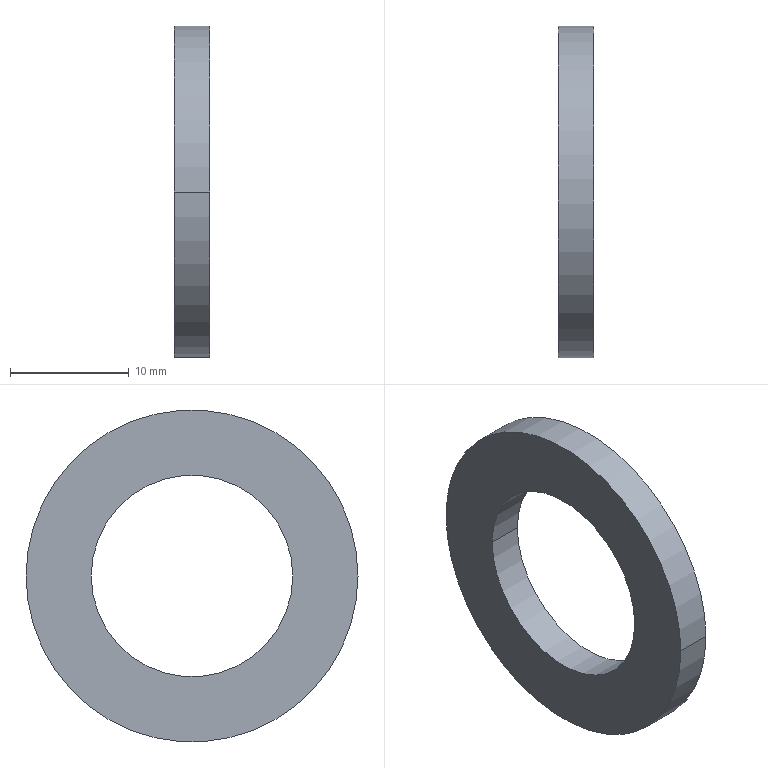Part | STEP file | KS B 1326 - 16x28 | 1 solid | 6 faces | box 3 x 28 x 28 mm | volume 1166 mm3 | cylinder 4 | plane 2 | commonest cylinder face diameters 17 x2 28 x2
STEP:
#1=CARTESIAN_POINT('',(0.,0.,0.));
#2=DIRECTION('',(0.,0.,1.));
#3=DIRECTION('',(1.,0.,0.));
#4=AXIS2_PLACEMENT_3D('',#1,#2,#3);
#5=CARTESIAN_POINT('',(0.,-8.5,0.));
#6=VERTEX_POINT('',#5);
#7=CARTESIAN_POINT('',(3.,-8.5,0.));
#8=VERTEX_POINT('',#7);
#9=CARTESIAN_POINT('',(0.,-8.5,0.));
#10=DIRECTION('',(1.,0.,0.));
#11=VECTOR('',#10,1.);
#12=LINE('',#9,#11);
#13=CARTESIAN_POINT('',(0.,0.,0.));
#14=DIRECTION('',(1.,0.,0.));
#15=DIRECTION('',(0.,-1.,0.));
#16=AXIS2_PLACEMENT_3D('',#13,#14,#15);
#17=CYLINDRICAL_SURFACE('',#16,8.5);
#18=CARTESIAN_POINT('',(6.283,0.));
#19=DIRECTION('',(0.,1.));
#20=VECTOR('',#19,1.);
#21=LINE('',#18,#20);
#22=(GEOMETRIC_REPRESENTATION_CONTEXT(2)PARAMETRIC_REPRESENTATION_CONTEXT()REPRESENTATION_CONTEXT('',''));
#23=DEFINITIONAL_REPRESENTATION('',(#21),#22);
#24=PCURVE('',#17,#23);
#25=CARTESIAN_POINT('',(0.,0.,0.));
#26=DIRECTION('',(1.,0.,0.));
#27=DIRECTION('',(0.,-1.,0.));
#28=AXIS2_PLACEMENT_3D('',#25,#26,#27);
#29=CYLINDRICAL_SURFACE('',#28,8.5);
#30=CARTESIAN_POINT('',(0.,0.));
#31=DIRECTION('',(0.,1.));
#32=VECTOR('',#31,1.);
#33=LINE('',#30,#32);
#34=(GEOMETRIC_REPRESENTATION_CONTEXT(2)PARAMETRIC_REPRESENTATION_CONTEXT()REPRESENTATION_CONTEXT('',''));
#35=DEFINITIONAL_REPRESENTATION('',(#33),#34);
#36=PCURVE('',#29,#35);
#37=SURFACE_CURVE('',#12,(#24,#36),.PCURVE_S1.);
#38=EDGE_CURVE('',#6,#8,#37,.T.);
#39=ORIENTED_EDGE('',*,*,#38,.T.);
#40=CARTESIAN_POINT('',(3.,8.5,0.));
#41=VERTEX_POINT('',#40);
#42=CARTESIAN_POINT('',(3.,0.,0.));
#43=DIRECTION('',(-1.,0.,0.));
#44=DIRECTION('',(0.,-1.,0.));
#45=AXIS2_PLACEMENT_3D('',#42,#43,#44);
#46=CIRCLE('',#45,8.5);
#47=CARTESIAN_POINT('',(6.283,3.));
#48=DIRECTION('',(-1.,0.));
#49=VECTOR('',#48,1.);
#50=LINE('',#47,#49);
#51=(GEOMETRIC_REPRESENTATION_CONTEXT(2)PARAMETRIC_REPRESENTATION_CONTEXT()REPRESENTATION_CONTEXT('',''));
#52=DEFINITIONAL_REPRESENTATION('',(#50),#51);
#53=PCURVE('',#17,#52);
#54=CARTESIAN_POINT('',(3.,0.,0.));
#55=DIRECTION('',(-1.,0.,0.));
#56=DIRECTION('',(0.,0.,1.));
#57=AXIS2_PLACEMENT_3D('',#54,#55,#56);
#58=PLANE('',#57);
#59=CARTESIAN_POINT('',(0.,0.));
#60=DIRECTION('',(0.,-1.));
#61=AXIS2_PLACEMENT_2D('',#59,#60);
#62=CIRCLE('',#61,8.5);
#63=(GEOMETRIC_REPRESENTATION_CONTEXT(2)PARAMETRIC_REPRESENTATION_CONTEXT()REPRESENTATION_CONTEXT('',''));
#64=DEFINITIONAL_REPRESENTATION('',(#62),#63);
#65=PCURVE('',#58,#64);
#66=SURFACE_CURVE('',#46,(#53,#65),.PCURVE_S1.);
#67=EDGE_CURVE('',#8,#41,#66,.T.);
#68=ORIENTED_EDGE('',*,*,#67,.T.);
#69=CARTESIAN_POINT('',(0.,8.5,0.));
#70=VERTEX_POINT('',#69);
#71=CARTESIAN_POINT('',(0.,8.5,0.));
#72=DIRECTION('',(1.,0.,0.));
#73=VECTOR('',#72,1.);
#74=LINE('',#71,#73);
#75=CARTESIAN_POINT('',(3.142,0.));
#76=DIRECTION('',(0.,1.));
#77=VECTOR('',#76,1.);
#78=LINE('',#75,#77);
#79=(GEOMETRIC_REPRESENTATION_CONTEXT(2)PARAMETRIC_REPRESENTATION_CONTEXT()REPRESENTATION_CONTEXT('',''));
#80=DEFINITIONAL_REPRESENTATION('',(#78),#79);
#81=PCURVE('',#17,#80);
#82=CARTESIAN_POINT('',(3.142,0.));
#83=DIRECTION('',(0.,1.));
#84=VECTOR('',#83,1.);
#85=LINE('',#82,#84);
#86=(GEOMETRIC_REPRESENTATION_CONTEXT(2)PARAMETRIC_REPRESENTATION_CONTEXT()REPRESENTATION_CONTEXT('',''));
#87=DEFINITIONAL_REPRESENTATION('',(#85),#86);
#88=PCURVE('',#29,#87);
#89=SURFACE_CURVE('',#74,(#81,#88),.PCURVE_S1.);
#90=EDGE_CURVE('',#70,#41,#89,.T.);
#91=ORIENTED_EDGE('',*,*,#90,.F.);
#92=CARTESIAN_POINT('',(0.,0.,0.));
#93=DIRECTION('',(1.,0.,0.));
#94=DIRECTION('',(0.,-1.,0.));
#95=AXIS2_PLACEMENT_3D('',#92,#93,#94);
#96=CIRCLE('',#95,8.5);
#97=CARTESIAN_POINT('',(0.,0.));
#98=DIRECTION('',(1.,0.));
#99=VECTOR('',#98,1.);
#100=LINE('',#97,#99);
#101=(GEOMETRIC_REPRESENTATION_CONTEXT(2)PARAMETRIC_REPRESENTATION_CONTEXT()REPRESENTATION_CONTEXT('',''));
#102=DEFINITIONAL_REPRESENTATION('',(#100),#101);
#103=PCURVE('',#17,#102);
#104=CARTESIAN_POINT('',(0.,0.,0.));
#105=DIRECTION('',(-1.,0.,0.));
#106=DIRECTION('',(0.,0.,1.));
#107=AXIS2_PLACEMENT_3D('',#104,#105,#106);
#108=PLANE('',#107);
#109=CARTESIAN_POINT('',(0.,-8.5));
#110=CARTESIAN_POINT('',(-14.722,-8.5));
#111=CARTESIAN_POINT('',(-7.361,4.25));
#112=CARTESIAN_POINT('',(0.,17.));
#113=CARTESIAN_POINT('',(7.361,4.25));
#114=CARTESIAN_POINT('',(14.722,-8.5));
#115=CARTESIAN_POINT('',(0.,-8.5));
#116=(BOUNDED_CURVE()B_SPLINE_CURVE(2,(#109,#110,#111,#112,#113,#114,#115),.UNSPECIFIED.,.T.,.F.)B_SPLINE_CURVE_WITH_KNOTS((1,2,2,2,2,1),(-2.094,0.,2.094,4.189,6.283,8.378),.UNSPECIFIED.)CURVE()GEOMETRIC_REPRESENTATION_ITEM()RATIONAL_B_SPLINE_CURVE((1.,0.5,1.,0.5,1.,0.5,1.))REPRESENTATION_ITEM(''));
#117=(GEOMETRIC_REPRESENTATION_CONTEXT(2)PARAMETRIC_REPRESENTATION_CONTEXT()REPRESENTATION_CONTEXT('',''));
#118=DEFINITIONAL_REPRESENTATION('',(#116),#117);
#119=PCURVE('',#108,#118);
#120=SURFACE_CURVE('',#96,(#103,#119),.PCURVE_S1.);
#121=EDGE_CURVE('',#70,#6,#120,.T.);
#122=ORIENTED_EDGE('',*,*,#121,.T.);
#123=EDGE_LOOP('',(#39,#68,#91,#122));
#124=FACE_BOUND('',#123,.F.);
#125=ADVANCED_FACE('',(#124),#17,.F.);
#126=CARTESIAN_POINT('',(0.,14.,0.));
#127=VERTEX_POINT('',#126);
#128=CARTESIAN_POINT('',(0.,-14.,0.));
#129=VERTEX_POINT('',#128);
#130=CARTESIAN_POINT('',(0.,0.,0.));
#131=DIRECTION('',(-1.,0.,0.));
#132=DIRECTION('',(0.,-1.,0.));
#133=AXIS2_PLACEMENT_3D('',#130,#131,#132);
#134=CIRCLE('',#133,14.);
#135=CARTESIAN_POINT('',(0.,0.,0.));
#136=DIRECTION('',(1.,0.,0.));
#137=DIRECTION('',(0.,-1.,0.));
#138=AXIS2_PLACEMENT_3D('',#135,#136,#137);
#139=CYLINDRICAL_SURFACE('',#138,14.);
#140=CARTESIAN_POINT('',(6.283,0.));
#141=DIRECTION('',(-1.,0.));
#142=VECTOR('',#141,1.);
#143=LINE('',#140,#142);
#144=(GEOMETRIC_REPRESENTATION_CONTEXT(2)PARAMETRIC_REPRESENTATION_CONTEXT()REPRESENTATION_CONTEXT('',''));
#145=DEFINITIONAL_REPRESENTATION('',(#143),#144);
#146=PCURVE('',#139,#145);
#147=CARTESIAN_POINT('',(0.,0.));
#148=DIRECTION('',(0.,-1.));
#149=AXIS2_PLACEMENT_2D('',#147,#148);
#150=CIRCLE('',#149,14.);
#151=(GEOMETRIC_REPRESENTATION_CONTEXT(2)PARAMETRIC_REPRESENTATION_CONTEXT()REPRESENTATION_CONTEXT('',''));
#152=DEFINITIONAL_REPRESENTATION('',(#150),#151);
#153=PCURVE('',#108,#152);
#154=SURFACE_CURVE('',#134,(#146,#153),.PCURVE_S1.);
#155=EDGE_CURVE('',#127,#129,#154,.T.);
#156=ORIENTED_EDGE('',*,*,#155,.F.);
#157=CARTESIAN_POINT('',(3.,14.,0.));
#158=VERTEX_POINT('',#157);
#159=CARTESIAN_POINT('',(0.,14.,0.));
#160=DIRECTION('',(1.,0.,0.));
#161=VECTOR('',#160,1.);
#162=LINE('',#159,#161);
#163=CARTESIAN_POINT('',(3.142,0.));
#164=DIRECTION('',(0.,1.));
#165=VECTOR('',#164,1.);
#166=LINE('',#163,#165);
#167=(GEOMETRIC_REPRESENTATION_CONTEXT(2)PARAMETRIC_REPRESENTATION_CONTEXT()REPRESENTATION_CONTEXT('',''));
#168=DEFINITIONAL_REPRESENTATION('',(#166),#167);
#169=PCURVE('',#139,#168);
#170=CARTESIAN_POINT('',(0.,0.,0.));
#171=DIRECTION('',(1.,0.,0.));
#172=DIRECTION('',(0.,-1.,0.));
#173=AXIS2_PLACEMENT_3D('',#170,#171,#172);
#174=CYLINDRICAL_SURFACE('',#173,14.);
#175=CARTESIAN_POINT('',(3.142,0.));
#176=DIRECTION('',(0.,1.));
#177=VECTOR('',#176,1.);
#178=LINE('',#175,#177);
#179=(GEOMETRIC_REPRESENTATION_CONTEXT(2)PARAMETRIC_REPRESENTATION_CONTEXT()REPRESENTATION_CONTEXT('',''));
#180=DEFINITIONAL_REPRESENTATION('',(#178),#179);
#181=PCURVE('',#174,#180);
#182=SURFACE_CURVE('',#162,(#169,#181),.PCURVE_S1.);
#183=EDGE_CURVE('',#127,#158,#182,.T.);
#184=ORIENTED_EDGE('',*,*,#183,.T.);
#185=CARTESIAN_POINT('',(3.,-14.,0.));
#186=VERTEX_POINT('',#185);
#187=CARTESIAN_POINT('',(3.,0.,0.));
#188=DIRECTION('',(-1.,0.,0.));
#189=DIRECTION('',(0.,-1.,0.));
#190=AXIS2_PLACEMENT_3D('',#187,#188,#189);
#191=CIRCLE('',#190,14.);
#192=CARTESIAN_POINT('',(6.283,3.));
#193=DIRECTION('',(-1.,0.));
#194=VECTOR('',#193,1.);
#195=LINE('',#192,#194);
#196=(GEOMETRIC_REPRESENTATION_CONTEXT(2)PARAMETRIC_REPRESENTATION_CONTEXT()REPRESENTATION_CONTEXT('',''));
#197=DEFINITIONAL_REPRESENTATION('',(#195),#196);
#198=PCURVE('',#139,#197);
#199=CARTESIAN_POINT('',(0.,0.));
#200=DIRECTION('',(0.,-1.));
#201=AXIS2_PLACEMENT_2D('',#199,#200);
#202=CIRCLE('',#201,14.);
#203=(GEOMETRIC_REPRESENTATION_CONTEXT(2)PARAMETRIC_REPRESENTATION_CONTEXT()REPRESENTATION_CONTEXT('',''));
#204=DEFINITIONAL_REPRESENTATION('',(#202),#203);
#205=PCURVE('',#58,#204);
#206=SURFACE_CURVE('',#191,(#198,#205),.PCURVE_S1.);
#207=EDGE_CURVE('',#158,#186,#206,.T.);
#208=ORIENTED_EDGE('',*,*,#207,.T.);
#209=CARTESIAN_POINT('',(0.,-14.,0.));
#210=DIRECTION('',(1.,0.,0.));
#211=VECTOR('',#210,1.);
#212=LINE('',#209,#211);
#213=CARTESIAN_POINT('',(0.,0.));
#214=DIRECTION('',(0.,1.));
#215=VECTOR('',#214,1.);
#216=LINE('',#213,#215);
#217=(GEOMETRIC_REPRESENTATION_CONTEXT(2)PARAMETRIC_REPRESENTATION_CONTEXT()REPRESENTATION_CONTEXT('',''));
#218=DEFINITIONAL_REPRESENTATION('',(#216),#217);
#219=PCURVE('',#139,#218);
#220=CARTESIAN_POINT('',(6.283,0.));
#221=DIRECTION('',(0.,1.));
#222=VECTOR('',#221,1.);
#223=LINE('',#220,#222);
#224=(GEOMETRIC_REPRESENTATION_CONTEXT(2)PARAMETRIC_REPRESENTATION_CONTEXT()REPRESENTATION_CONTEXT('',''));
#225=DEFINITIONAL_REPRESENTATION('',(#223),#224);
#226=PCURVE('',#174,#225);
#227=SURFACE_CURVE('',#212,(#219,#226),.PCURVE_S1.);
#228=EDGE_CURVE('',#129,#186,#227,.T.);
#229=ORIENTED_EDGE('',*,*,#228,.F.);
#230=EDGE_LOOP('',(#156,#184,#208,#229));
#231=FACE_BOUND('',#230,.T.);
#232=ADVANCED_FACE('',(#231),#139,.T.);
#233=CARTESIAN_POINT('',(0.,0.,0.));
#234=DIRECTION('',(1.,0.,0.));
#235=DIRECTION('',(0.,-1.,0.));
#236=AXIS2_PLACEMENT_3D('',#233,#234,#235);
#237=CIRCLE('',#236,8.5);
#238=CARTESIAN_POINT('',(0.,-8.5));
#239=CARTESIAN_POINT('',(-14.722,-8.5));
#240=CARTESIAN_POINT('',(-7.361,4.25));
#241=CARTESIAN_POINT('',(0.,17.));
#242=CARTESIAN_POINT('',(7.361,4.25));
#243=CARTESIAN_POINT('',(14.722,-8.5));
#244=CARTESIAN_POINT('',(0.,-8.5));
#245=(BOUNDED_CURVE()B_SPLINE_CURVE(2,(#238,#239,#240,#241,#242,#243,#244),.UNSPECIFIED.,.T.,.F.)B_SPLINE_CURVE_WITH_KNOTS((1,2,2,2,2,1),(-2.094,0.,2.094,4.189,6.283,8.378),.UNSPECIFIED.)CURVE()GEOMETRIC_REPRESENTATION_ITEM()RATIONAL_B_SPLINE_CURVE((1.,0.5,1.,0.5,1.,0.5,1.))REPRESENTATION_ITEM(''));
#246=(GEOMETRIC_REPRESENTATION_CONTEXT(2)PARAMETRIC_REPRESENTATION_CONTEXT()REPRESENTATION_CONTEXT('',''));
#247=DEFINITIONAL_REPRESENTATION('',(#245),#246);
#248=PCURVE('',#108,#247);
#249=CARTESIAN_POINT('',(0.,0.));
#250=DIRECTION('',(1.,0.));
#251=VECTOR('',#250,1.);
#252=LINE('',#249,#251);
#253=(GEOMETRIC_REPRESENTATION_CONTEXT(2)PARAMETRIC_REPRESENTATION_CONTEXT()REPRESENTATION_CONTEXT('',''));
#254=DEFINITIONAL_REPRESENTATION('',(#252),#253);
#255=PCURVE('',#29,#254);
#256=SURFACE_CURVE('',#237,(#248,#255),.PCURVE_S1.);
#257=EDGE_CURVE('',#6,#70,#256,.T.);
#258=ORIENTED_EDGE('',*,*,#257,.T.);
#259=ORIENTED_EDGE('',*,*,#121,.T.);
#260=EDGE_LOOP('',(#258,#259));
#261=FACE_BOUND('',#260,.T.);
#262=CARTESIAN_POINT('',(0.,0.,0.));
#263=DIRECTION('',(-1.,0.,0.));
#264=DIRECTION('',(0.,-1.,0.));
#265=AXIS2_PLACEMENT_3D('',#262,#263,#264);
#266=CIRCLE('',#265,14.);
#267=CARTESIAN_POINT('',(0.,0.));
#268=DIRECTION('',(0.,-1.));
#269=AXIS2_PLACEMENT_2D('',#267,#268);
#270=CIRCLE('',#269,14.);
#271=(GEOMETRIC_REPRESENTATION_CONTEXT(2)PARAMETRIC_REPRESENTATION_CONTEXT()REPRESENTATION_CONTEXT('',''));
#272=DEFINITIONAL_REPRESENTATION('',(#270),#271);
#273=PCURVE('',#108,#272);
#274=CARTESIAN_POINT('',(6.283,0.));
#275=DIRECTION('',(-1.,0.));
#276=VECTOR('',#275,1.);
#277=LINE('',#274,#276);
#278=(GEOMETRIC_REPRESENTATION_CONTEXT(2)PARAMETRIC_REPRESENTATION_CONTEXT()REPRESENTATION_CONTEXT('',''));
#279=DEFINITIONAL_REPRESENTATION('',(#277),#278);
#280=PCURVE('',#174,#279);
#281=SURFACE_CURVE('',#266,(#273,#280),.PCURVE_S1.);
#282=EDGE_CURVE('',#129,#127,#281,.T.);
#283=ORIENTED_EDGE('',*,*,#282,.T.);
#284=ORIENTED_EDGE('',*,*,#155,.T.);
#285=EDGE_LOOP('',(#283,#284));
#286=FACE_BOUND('',#285,.T.);
#287=ADVANCED_FACE('',(#261,#286),#108,.T.);
#288=ORIENTED_EDGE('',*,*,#67,.T.);
#289=CARTESIAN_POINT('',(3.,0.,0.));
#290=DIRECTION('',(-1.,0.,0.));
#291=DIRECTION('',(0.,-1.,0.));
#292=AXIS2_PLACEMENT_3D('',#289,#290,#291);
#293=CIRCLE('',#292,8.5);
#294=CARTESIAN_POINT('',(0.,0.));
#295=DIRECTION('',(0.,-1.));
#296=AXIS2_PLACEMENT_2D('',#294,#295);
#297=CIRCLE('',#296,8.5);
#298=(GEOMETRIC_REPRESENTATION_CONTEXT(2)PARAMETRIC_REPRESENTATION_CONTEXT()REPRESENTATION_CONTEXT('',''));
#299=DEFINITIONAL_REPRESENTATION('',(#297),#298);
#300=PCURVE('',#58,#299);
#301=CARTESIAN_POINT('',(6.283,3.));
#302=DIRECTION('',(-1.,0.));
#303=VECTOR('',#302,1.);
#304=LINE('',#301,#303);
#305=(GEOMETRIC_REPRESENTATION_CONTEXT(2)PARAMETRIC_REPRESENTATION_CONTEXT()REPRESENTATION_CONTEXT('',''));
#306=DEFINITIONAL_REPRESENTATION('',(#304),#305);
#307=PCURVE('',#29,#306);
#308=SURFACE_CURVE('',#293,(#300,#307),.PCURVE_S1.);
#309=EDGE_CURVE('',#41,#8,#308,.T.);
#310=ORIENTED_EDGE('',*,*,#309,.T.);
#311=EDGE_LOOP('',(#288,#310));
#312=FACE_BOUND('',#311,.T.);
#313=CARTESIAN_POINT('',(3.,0.,0.));
#314=DIRECTION('',(-1.,0.,0.));
#315=DIRECTION('',(0.,-1.,0.));
#316=AXIS2_PLACEMENT_3D('',#313,#314,#315);
#317=CIRCLE('',#316,14.);
#318=CARTESIAN_POINT('',(0.,0.));
#319=DIRECTION('',(0.,-1.));
#320=AXIS2_PLACEMENT_2D('',#318,#319);
#321=CIRCLE('',#320,14.);
#322=(GEOMETRIC_REPRESENTATION_CONTEXT(2)PARAMETRIC_REPRESENTATION_CONTEXT()REPRESENTATION_CONTEXT('',''));
#323=DEFINITIONAL_REPRESENTATION('',(#321),#322);
#324=PCURVE('',#58,#323);
#325=CARTESIAN_POINT('',(6.283,3.));
#326=DIRECTION('',(-1.,0.));
#327=VECTOR('',#326,1.);
#328=LINE('',#325,#327);
#329=(GEOMETRIC_REPRESENTATION_CONTEXT(2)PARAMETRIC_REPRESENTATION_CONTEXT()REPRESENTATION_CONTEXT('',''));
#330=DEFINITIONAL_REPRESENTATION('',(#328),#329);
#331=PCURVE('',#174,#330);
#332=SURFACE_CURVE('',#317,(#324,#331),.PCURVE_S1.);
#333=EDGE_CURVE('',#186,#158,#332,.T.);
#334=ORIENTED_EDGE('',*,*,#333,.F.);
#335=ORIENTED_EDGE('',*,*,#207,.F.);
#336=EDGE_LOOP('',(#334,#335));
#337=FACE_BOUND('',#336,.T.);
#338=ADVANCED_FACE('',(#312,#337),#58,.F.);
#339=ORIENTED_EDGE('',*,*,#183,.F.);
#340=ORIENTED_EDGE('',*,*,#282,.F.);
#341=ORIENTED_EDGE('',*,*,#228,.T.);
#342=ORIENTED_EDGE('',*,*,#333,.T.);
#343=EDGE_LOOP('',(#339,#340,#341,#342));
#344=FACE_BOUND('',#343,.T.);
#345=ADVANCED_FACE('',(#344),#174,.T.);
#346=ORIENTED_EDGE('',*,*,#309,.T.);
#347=ORIENTED_EDGE('',*,*,#38,.F.);
#348=ORIENTED_EDGE('',*,*,#257,.T.);
#349=ORIENTED_EDGE('',*,*,#90,.T.);
#350=EDGE_LOOP('',(#346,#347,#348,#349));
#351=FACE_BOUND('',#350,.F.);
#352=ADVANCED_FACE('',(#351),#29,.F.);
#353=CLOSED_SHELL('',(#125,#232,#287,#338,#345,#352));
#354=MANIFOLD_SOLID_BREP('',#353);
#355=(LENGTH_UNIT()NAMED_UNIT(*)SI_UNIT(.MILLI.,.METRE.));
#356=UNCERTAINTY_MEASURE_WITH_UNIT(LENGTH_MEASURE(0.0000001),#355,'','');
#357=(NAMED_UNIT(*)PLANE_ANGLE_UNIT()SI_UNIT($,.RADIAN.));
#358=(NAMED_UNIT(*)SI_UNIT($,.STERADIAN.)SOLID_ANGLE_UNIT());
#359=(GEOMETRIC_REPRESENTATION_CONTEXT(3)GLOBAL_UNCERTAINTY_ASSIGNED_CONTEXT((#356))GLOBAL_UNIT_ASSIGNED_CONTEXT((#355,#357,#358))REPRESENTATION_CONTEXT('',''));
#360=ADVANCED_BREP_SHAPE_REPRESENTATION('',(#4,#354),#359);